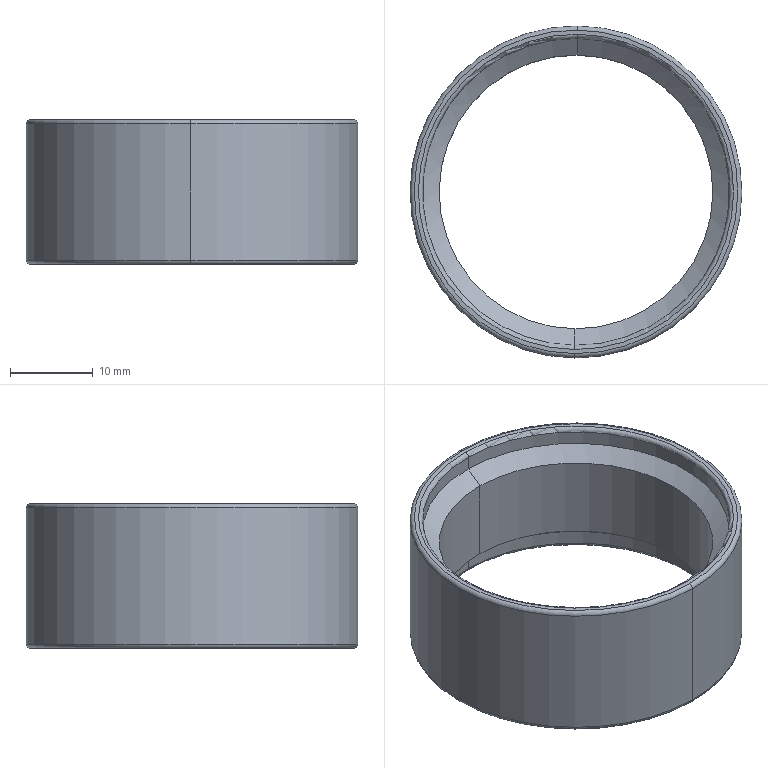Part | SolidWorks | features SplitBody 1 | 1 solid | 22 faces | box 40 x 40 x 17.4 mm | volume 5666 mm3 | cylinder 8 | torus 8 | cone 4 | plane 2 | commonest cylinder face diameters 37 x4 33 x2 40 x2
STEP:
#1=CARTESIAN_POINT('',(540.428,13.025,-486.947));
#2=VERTEX_POINT('',#1);
#3=CARTESIAN_POINT('',(540.156,-23.974,-486.947));
#4=VERTEX_POINT('',#3);
#5=CARTESIAN_POINT('',(540.292,-5.475,-486.947));
#6=DIRECTION('',(0.,0.,1.));
#7=DIRECTION('',(-0.00734,-1.,0.));
#8=AXIS2_PLACEMENT_3D('',#5,#6,#7);
#9=CIRCLE('',#8,18.5);
#10=EDGE_CURVE('',#2,#4,#9,.T.);
#11=ORIENTED_EDGE('',*,*,#10,.F.);
#12=CARTESIAN_POINT('',(540.428,13.025,-485.247));
#13=VERTEX_POINT('',#12);
#14=CARTESIAN_POINT('',(540.428,13.025,-478.747));
#15=DIRECTION('',(0.,0.,1.));
#16=VECTOR('',#15,1000.);
#17=LINE('',#14,#16);
#18=EDGE_CURVE('',#2,#13,#17,.T.);
#19=ORIENTED_EDGE('',*,*,#18,.T.);
#20=CARTESIAN_POINT('',(540.156,-23.974,-485.247));
#21=VERTEX_POINT('',#20);
#22=CARTESIAN_POINT('',(540.292,-5.475,-485.247));
#23=DIRECTION('',(0.,0.,1.));
#24=DIRECTION('',(-0.00734,-1.,0.));
#25=AXIS2_PLACEMENT_3D('',#22,#23,#24);
#26=CIRCLE('',#25,18.5);
#27=EDGE_CURVE('',#13,#21,#26,.T.);
#28=ORIENTED_EDGE('',*,*,#27,.T.);
#29=CARTESIAN_POINT('',(540.156,-23.974,-478.747));
#30=DIRECTION('',(0.,0.,1.));
#31=VECTOR('',#30,1000.);
#32=LINE('',#29,#31);
#33=EDGE_CURVE('',#4,#21,#32,.T.);
#34=ORIENTED_EDGE('',*,*,#33,.F.);
#35=EDGE_LOOP('',(#11,#19,#28,#34));
#36=FACE_OUTER_BOUND('',#35,.T.);
#37=CARTESIAN_POINT('',(540.292,-5.475,-478.747));
#38=DIRECTION('',(0.,0.,1.));
#39=DIRECTION('',(-0.00734,-1.,0.));
#40=AXIS2_PLACEMENT_3D('',#37,#38,#39);
#41=CYLINDRICAL_SURFACE('',#40,18.5);
#42=ADVANCED_FACE('',(#36),#41,.F.);
#43=CARTESIAN_POINT('',(540.292,-5.475,-486.947));
#44=DIRECTION('',(0.,0.,1.));
#45=DIRECTION('',(-0.00734,-1.,0.));
#46=AXIS2_PLACEMENT_3D('',#43,#44,#45);
#47=CIRCLE('',#46,18.5);
#48=EDGE_CURVE('',#4,#2,#47,.T.);
#49=ORIENTED_EDGE('',*,*,#48,.T.);
#50=CARTESIAN_POINT('',(540.432,13.525,-487.447));
#51=VERTEX_POINT('',#50);
#52=CARTESIAN_POINT('',(540.432,13.525,-486.947));
#53=DIRECTION('',(1.,-0.00734,0.));
#54=DIRECTION('',(0.00734,1.,0.));
#55=AXIS2_PLACEMENT_3D('',#52,#53,#54);
#56=CIRCLE('',#55,0.5);
#57=EDGE_CURVE('',#2,#51,#56,.T.);
#58=ORIENTED_EDGE('',*,*,#57,.T.);
#59=CARTESIAN_POINT('',(540.153,-24.474,-487.447));
#60=VERTEX_POINT('',#59);
#61=CARTESIAN_POINT('',(540.292,-5.475,-487.447));
#62=DIRECTION('',(0.,0.,1.));
#63=DIRECTION('',(-0.00734,-1.,0.));
#64=AXIS2_PLACEMENT_3D('',#61,#62,#63);
#65=CIRCLE('',#64,19.);
#66=EDGE_CURVE('',#60,#51,#65,.T.);
#67=ORIENTED_EDGE('',*,*,#66,.F.);
#68=CARTESIAN_POINT('',(540.153,-24.474,-486.947));
#69=DIRECTION('',(-1.,0.00734,0.));
#70=DIRECTION('',(-0.00734,-1.,0.));
#71=AXIS2_PLACEMENT_3D('',#68,#69,#70);
#72=CIRCLE('',#71,0.5);
#73=EDGE_CURVE('',#4,#60,#72,.T.);
#74=ORIENTED_EDGE('',*,*,#73,.F.);
#75=EDGE_LOOP('',(#49,#58,#67,#74));
#76=FACE_OUTER_BOUND('',#75,.T.);
#77=CARTESIAN_POINT('',(540.292,-5.475,-486.947));
#78=DIRECTION('',(0.,0.,1.));
#79=DIRECTION('',(-0.00734,-1.,0.));
#80=AXIS2_PLACEMENT_3D('',#77,#78,#79);
#81=TOROIDAL_SURFACE('',#80,19.,0.5);
#82=ADVANCED_FACE('',(#76),#81,.T.);
#83=CARTESIAN_POINT('',(540.149,-24.974,-487.447));
#84=VERTEX_POINT('',#83);
#85=CARTESIAN_POINT('',(540.435,14.025,-487.447));
#86=VERTEX_POINT('',#85);
#87=CARTESIAN_POINT('',(540.292,-5.475,-487.447));
#88=DIRECTION('',(0.,0.,1.));
#89=DIRECTION('',(-0.00734,-1.,0.));
#90=AXIS2_PLACEMENT_3D('',#87,#88,#89);
#91=CIRCLE('',#90,19.5);
#92=EDGE_CURVE('',#84,#86,#91,.T.);
#93=ORIENTED_EDGE('',*,*,#92,.T.);
#94=CARTESIAN_POINT('',(540.439,14.525,-486.947));
#95=VERTEX_POINT('',#94);
#96=CARTESIAN_POINT('',(540.435,14.025,-486.947));
#97=DIRECTION('',(1.,-0.00734,0.));
#98=DIRECTION('',(0.00734,1.,0.));
#99=AXIS2_PLACEMENT_3D('',#96,#97,#98);
#100=CIRCLE('',#99,0.5);
#101=EDGE_CURVE('',#86,#95,#100,.T.);
#102=ORIENTED_EDGE('',*,*,#101,.T.);
#103=CARTESIAN_POINT('',(540.145,-25.474,-486.947));
#104=VERTEX_POINT('',#103);
#105=CARTESIAN_POINT('',(540.292,-5.475,-486.947));
#106=DIRECTION('',(0.,0.,1.));
#107=DIRECTION('',(-0.00734,-1.,0.));
#108=AXIS2_PLACEMENT_3D('',#105,#106,#107);
#109=CIRCLE('',#108,20.);
#110=EDGE_CURVE('',#104,#95,#109,.T.);
#111=ORIENTED_EDGE('',*,*,#110,.F.);
#112=CARTESIAN_POINT('',(540.149,-24.974,-486.947));
#113=DIRECTION('',(-1.,0.00734,0.));
#114=DIRECTION('',(-0.00734,-1.,0.));
#115=AXIS2_PLACEMENT_3D('',#112,#113,#114);
#116=CIRCLE('',#115,0.5);
#117=EDGE_CURVE('',#84,#104,#116,.T.);
#118=ORIENTED_EDGE('',*,*,#117,.F.);
#119=EDGE_LOOP('',(#93,#102,#111,#118));
#120=FACE_OUTER_BOUND('',#119,.T.);
#121=CARTESIAN_POINT('',(540.292,-5.475,-486.947));
#122=DIRECTION('',(0.,0.,1.));
#123=DIRECTION('',(-0.00734,-1.,0.));
#124=AXIS2_PLACEMENT_3D('',#121,#122,#123);
#125=TOROIDAL_SURFACE('',#124,19.5,0.5);
#126=ADVANCED_FACE('',(#120),#125,.T.);
#127=ORIENTED_EDGE('',*,*,#110,.T.);
#128=CARTESIAN_POINT('',(540.439,14.525,-470.547));
#129=VERTEX_POINT('',#128);
#130=CARTESIAN_POINT('',(540.439,14.525,-478.747));
#131=DIRECTION('',(0.,0.,1.));
#132=VECTOR('',#131,1000.);
#133=LINE('',#130,#132);
#134=EDGE_CURVE('',#95,#129,#133,.T.);
#135=ORIENTED_EDGE('',*,*,#134,.T.);
#136=CARTESIAN_POINT('',(540.145,-25.474,-470.547));
#137=VERTEX_POINT('',#136);
#138=CARTESIAN_POINT('',(540.292,-5.475,-470.547));
#139=DIRECTION('',(0.,0.,1.));
#140=DIRECTION('',(-0.00734,-1.,0.));
#141=AXIS2_PLACEMENT_3D('',#138,#139,#140);
#142=CIRCLE('',#141,20.);
#143=EDGE_CURVE('',#137,#129,#142,.T.);
#144=ORIENTED_EDGE('',*,*,#143,.F.);
#145=CARTESIAN_POINT('',(540.145,-25.474,-478.747));
#146=DIRECTION('',(0.,0.,1.));
#147=VECTOR('',#146,1000.);
#148=LINE('',#145,#147);
#149=EDGE_CURVE('',#104,#137,#148,.T.);
#150=ORIENTED_EDGE('',*,*,#149,.F.);
#151=EDGE_LOOP('',(#127,#135,#144,#150));
#152=FACE_OUTER_BOUND('',#151,.T.);
#153=CARTESIAN_POINT('',(540.292,-5.475,-478.747));
#154=DIRECTION('',(0.,0.,1.));
#155=DIRECTION('',(-0.00734,-1.,0.));
#156=AXIS2_PLACEMENT_3D('',#153,#154,#155);
#157=CYLINDRICAL_SURFACE('',#156,20.);
#158=ADVANCED_FACE('',(#152),#157,.T.);
#159=ORIENTED_EDGE('',*,*,#143,.T.);
#160=CARTESIAN_POINT('',(540.435,14.025,-470.047));
#161=VERTEX_POINT('',#160);
#162=CARTESIAN_POINT('',(540.435,14.025,-470.547));
#163=DIRECTION('',(1.,-0.00734,0.));
#164=DIRECTION('',(0.00734,1.,0.));
#165=AXIS2_PLACEMENT_3D('',#162,#163,#164);
#166=CIRCLE('',#165,0.5);
#167=EDGE_CURVE('',#129,#161,#166,.T.);
#168=ORIENTED_EDGE('',*,*,#167,.T.);
#169=CARTESIAN_POINT('',(540.149,-24.974,-470.047));
#170=VERTEX_POINT('',#169);
#171=CARTESIAN_POINT('',(540.292,-5.475,-470.047));
#172=DIRECTION('',(0.,0.,1.));
#173=DIRECTION('',(-0.00734,-1.,0.));
#174=AXIS2_PLACEMENT_3D('',#171,#172,#173);
#175=CIRCLE('',#174,19.5);
#176=EDGE_CURVE('',#170,#161,#175,.T.);
#177=ORIENTED_EDGE('',*,*,#176,.F.);
#178=CARTESIAN_POINT('',(540.149,-24.974,-470.547));
#179=DIRECTION('',(-1.,0.00734,0.));
#180=DIRECTION('',(-0.00734,-1.,0.));
#181=AXIS2_PLACEMENT_3D('',#178,#179,#180);
#182=CIRCLE('',#181,0.5);
#183=EDGE_CURVE('',#137,#170,#182,.T.);
#184=ORIENTED_EDGE('',*,*,#183,.F.);
#185=EDGE_LOOP('',(#159,#168,#177,#184));
#186=FACE_OUTER_BOUND('',#185,.T.);
#187=CARTESIAN_POINT('',(540.292,-5.475,-470.547));
#188=DIRECTION('',(0.,0.,1.));
#189=DIRECTION('',(-0.00734,-1.,0.));
#190=AXIS2_PLACEMENT_3D('',#187,#188,#189);
#191=TOROIDAL_SURFACE('',#190,19.5,0.5);
#192=ADVANCED_FACE('',(#186),#191,.T.);
#193=CARTESIAN_POINT('',(540.153,-24.474,-470.047));
#194=VERTEX_POINT('',#193);
#195=CARTESIAN_POINT('',(540.432,13.525,-470.047));
#196=VERTEX_POINT('',#195);
#197=CARTESIAN_POINT('',(540.292,-5.475,-470.047));
#198=DIRECTION('',(0.,0.,1.));
#199=DIRECTION('',(-0.00734,-1.,0.));
#200=AXIS2_PLACEMENT_3D('',#197,#198,#199);
#201=CIRCLE('',#200,19.);
#202=EDGE_CURVE('',#194,#196,#201,.T.);
#203=ORIENTED_EDGE('',*,*,#202,.T.);
#204=CARTESIAN_POINT('',(540.428,13.025,-470.547));
#205=VERTEX_POINT('',#204);
#206=CARTESIAN_POINT('',(540.432,13.525,-470.547));
#207=DIRECTION('',(1.,-0.00734,0.));
#208=DIRECTION('',(0.00734,1.,0.));
#209=AXIS2_PLACEMENT_3D('',#206,#207,#208);
#210=CIRCLE('',#209,0.5);
#211=EDGE_CURVE('',#196,#205,#210,.T.);
#212=ORIENTED_EDGE('',*,*,#211,.T.);
#213=CARTESIAN_POINT('',(540.156,-23.974,-470.547));
#214=VERTEX_POINT('',#213);
#215=CARTESIAN_POINT('',(540.292,-5.475,-470.547));
#216=DIRECTION('',(0.,0.,1.));
#217=DIRECTION('',(-0.00734,-1.,0.));
#218=AXIS2_PLACEMENT_3D('',#215,#216,#217);
#219=CIRCLE('',#218,18.5);
#220=EDGE_CURVE('',#214,#205,#219,.T.);
#221=ORIENTED_EDGE('',*,*,#220,.F.);
#222=CARTESIAN_POINT('',(540.153,-24.474,-470.547));
#223=DIRECTION('',(-1.,0.00734,0.));
#224=DIRECTION('',(-0.00734,-1.,0.));
#225=AXIS2_PLACEMENT_3D('',#222,#223,#224);
#226=CIRCLE('',#225,0.5);
#227=EDGE_CURVE('',#194,#214,#226,.T.);
#228=ORIENTED_EDGE('',*,*,#227,.F.);
#229=EDGE_LOOP('',(#203,#212,#221,#228));
#230=FACE_OUTER_BOUND('',#229,.T.);
#231=CARTESIAN_POINT('',(540.292,-5.475,-470.547));
#232=DIRECTION('',(0.,0.,1.));
#233=DIRECTION('',(-0.00734,-1.,0.));
#234=AXIS2_PLACEMENT_3D('',#231,#232,#233);
#235=TOROIDAL_SURFACE('',#234,19.,0.5);
#236=ADVANCED_FACE('',(#230),#235,.T.);
#237=CARTESIAN_POINT('',(540.428,13.025,-472.247));
#238=VERTEX_POINT('',#237);
#239=CARTESIAN_POINT('',(540.156,-23.974,-472.247));
#240=VERTEX_POINT('',#239);
#241=CARTESIAN_POINT('',(540.292,-5.475,-472.247));
#242=DIRECTION('',(0.,0.,1.));
#243=DIRECTION('',(-0.00734,-1.,0.));
#244=AXIS2_PLACEMENT_3D('',#241,#242,#243);
#245=CIRCLE('',#244,18.5);
#246=EDGE_CURVE('',#238,#240,#245,.T.);
#247=ORIENTED_EDGE('',*,*,#246,.F.);
#248=CARTESIAN_POINT('',(540.428,13.025,-478.747));
#249=DIRECTION('',(0.,0.,1.));
#250=VECTOR('',#249,1000.);
#251=LINE('',#248,#250);
#252=EDGE_CURVE('',#238,#205,#251,.T.);
#253=ORIENTED_EDGE('',*,*,#252,.T.);
#254=CARTESIAN_POINT('',(540.292,-5.475,-470.547));
#255=DIRECTION('',(0.,0.,1.));
#256=DIRECTION('',(-0.00734,-1.,0.));
#257=AXIS2_PLACEMENT_3D('',#254,#255,#256);
#258=CIRCLE('',#257,18.5);
#259=EDGE_CURVE('',#205,#214,#258,.T.);
#260=ORIENTED_EDGE('',*,*,#259,.T.);
#261=CARTESIAN_POINT('',(540.156,-23.974,-478.747));
#262=DIRECTION('',(0.,0.,1.));
#263=VECTOR('',#262,1000.);
#264=LINE('',#261,#263);
#265=EDGE_CURVE('',#240,#214,#264,.T.);
#266=ORIENTED_EDGE('',*,*,#265,.F.);
#267=EDGE_LOOP('',(#247,#253,#260,#266));
#268=FACE_OUTER_BOUND('',#267,.T.);
#269=CARTESIAN_POINT('',(540.292,-5.475,-478.747));
#270=DIRECTION('',(0.,0.,1.));
#271=DIRECTION('',(-0.00734,-1.,0.));
#272=AXIS2_PLACEMENT_3D('',#269,#270,#271);
#273=CYLINDRICAL_SURFACE('',#272,18.5);
#274=ADVANCED_FACE('',(#268),#273,.F.);
#275=CARTESIAN_POINT('',(540.413,11.025,-473.747));
#276=VERTEX_POINT('',#275);
#277=CARTESIAN_POINT('',(540.171,-21.974,-473.747));
#278=VERTEX_POINT('',#277);
#279=CARTESIAN_POINT('',(540.292,-5.475,-473.747));
#280=DIRECTION('',(0.,0.,1.));
#281=DIRECTION('',(-0.00734,-1.,0.));
#282=AXIS2_PLACEMENT_3D('',#279,#280,#281);
#283=CIRCLE('',#282,16.5);
#284=EDGE_CURVE('',#276,#278,#283,.T.);
#285=ORIENTED_EDGE('',*,*,#284,.F.);
#286=CARTESIAN_POINT('',(540.413,11.025,-473.747));
#287=DIRECTION('',(0.005872,0.8,0.6));
#288=VECTOR('',#287,1000.);
#289=LINE('',#286,#288);
#290=EDGE_CURVE('',#276,#238,#289,.T.);
#291=ORIENTED_EDGE('',*,*,#290,.T.);
#292=ORIENTED_EDGE('',*,*,#246,.T.);
#293=CARTESIAN_POINT('',(540.171,-21.974,-473.747));
#294=DIRECTION('',(-0.005872,-0.8,0.6));
#295=VECTOR('',#294,1000.);
#296=LINE('',#293,#295);
#297=EDGE_CURVE('',#278,#240,#296,.T.);
#298=ORIENTED_EDGE('',*,*,#297,.F.);
#299=EDGE_LOOP('',(#285,#291,#292,#298));
#300=FACE_OUTER_BOUND('',#299,.T.);
#301=CARTESIAN_POINT('',(540.292,-5.475,-473.747));
#302=DIRECTION('',(0.,0.,1.));
#303=DIRECTION('',(-0.00734,-1.,0.));
#304=AXIS2_PLACEMENT_3D('',#301,#302,#303);
#305=CONICAL_SURFACE('',#304,16.5,0.9273);
#306=ADVANCED_FACE('',(#300),#305,.F.);
#307=CARTESIAN_POINT('',(540.413,11.025,-483.747));
#308=VERTEX_POINT('',#307);
#309=CARTESIAN_POINT('',(540.171,-21.974,-483.747));
#310=VERTEX_POINT('',#309);
#311=CARTESIAN_POINT('',(540.292,-5.475,-483.747));
#312=DIRECTION('',(0.,0.,1.));
#313=DIRECTION('',(-0.00734,-1.,0.));
#314=AXIS2_PLACEMENT_3D('',#311,#312,#313);
#315=CIRCLE('',#314,16.5);
#316=EDGE_CURVE('',#308,#310,#315,.T.);
#317=ORIENTED_EDGE('',*,*,#316,.F.);
#318=CARTESIAN_POINT('',(540.413,11.025,-478.747));
#319=DIRECTION('',(0.,0.,1.));
#320=VECTOR('',#319,1000.);
#321=LINE('',#318,#320);
#322=EDGE_CURVE('',#308,#276,#321,.T.);
#323=ORIENTED_EDGE('',*,*,#322,.T.);
#324=ORIENTED_EDGE('',*,*,#284,.T.);
#325=CARTESIAN_POINT('',(540.171,-21.974,-478.747));
#326=DIRECTION('',(0.,0.,1.));
#327=VECTOR('',#326,1000.);
#328=LINE('',#325,#327);
#329=EDGE_CURVE('',#310,#278,#328,.T.);
#330=ORIENTED_EDGE('',*,*,#329,.F.);
#331=EDGE_LOOP('',(#317,#323,#324,#330));
#332=FACE_OUTER_BOUND('',#331,.T.);
#333=CARTESIAN_POINT('',(540.292,-5.475,-478.747));
#334=DIRECTION('',(0.,0.,1.));
#335=DIRECTION('',(-0.00734,-1.,0.));
#336=AXIS2_PLACEMENT_3D('',#333,#334,#335);
#337=CYLINDRICAL_SURFACE('',#336,16.5);
#338=ADVANCED_FACE('',(#332),#337,.F.);
#339=ORIENTED_EDGE('',*,*,#316,.T.);
#340=CARTESIAN_POINT('',(540.156,-23.974,-485.247));
#341=DIRECTION('',(-0.005872,-0.8,-0.6));
#342=VECTOR('',#341,1000.);
#343=LINE('',#340,#342);
#344=EDGE_CURVE('',#310,#21,#343,.T.);
#345=ORIENTED_EDGE('',*,*,#344,.T.);
#346=ORIENTED_EDGE('',*,*,#27,.F.);
#347=CARTESIAN_POINT('',(540.428,13.025,-485.247));
#348=DIRECTION('',(0.005872,0.8,-0.6));
#349=VECTOR('',#348,1000.);
#350=LINE('',#347,#349);
#351=EDGE_CURVE('',#308,#13,#350,.T.);
#352=ORIENTED_EDGE('',*,*,#351,.F.);
#353=EDGE_LOOP('',(#339,#345,#346,#352));
#354=FACE_OUTER_BOUND('',#353,.T.);
#355=CARTESIAN_POINT('',(540.292,-5.475,-485.247));
#356=DIRECTION('',(0.,0.,-1.));
#357=DIRECTION('',(0.00734,1.,0.));
#358=AXIS2_PLACEMENT_3D('',#355,#356,#357);
#359=CONICAL_SURFACE('',#358,18.5,0.9273);
#360=ADVANCED_FACE('',(#354),#359,.F.);
#361=ORIENTED_EDGE('',*,*,#344,.F.);
#362=CARTESIAN_POINT('',(540.292,-5.475,-483.747));
#363=DIRECTION('',(0.,0.,1.));
#364=DIRECTION('',(-0.00734,-1.,0.));
#365=AXIS2_PLACEMENT_3D('',#362,#363,#364);
#366=CIRCLE('',#365,16.5);
#367=EDGE_CURVE('',#310,#308,#366,.T.);
#368=ORIENTED_EDGE('',*,*,#367,.T.);
#369=ORIENTED_EDGE('',*,*,#351,.T.);
#370=CARTESIAN_POINT('',(540.292,-5.475,-485.247));
#371=DIRECTION('',(0.,0.,1.));
#372=DIRECTION('',(-0.00734,-1.,0.));
#373=AXIS2_PLACEMENT_3D('',#370,#371,#372);
#374=CIRCLE('',#373,18.5);
#375=EDGE_CURVE('',#21,#13,#374,.T.);
#376=ORIENTED_EDGE('',*,*,#375,.F.);
#377=EDGE_LOOP('',(#361,#368,#369,#376));
#378=FACE_OUTER_BOUND('',#377,.T.);
#379=CARTESIAN_POINT('',(540.292,-5.475,-485.247));
#380=DIRECTION('',(0.,0.,-1.));
#381=DIRECTION('',(0.00734,1.,0.));
#382=AXIS2_PLACEMENT_3D('',#379,#380,#381);
#383=CONICAL_SURFACE('',#382,18.5,0.9273);
#384=ADVANCED_FACE('',(#378),#383,.F.);
#385=ORIENTED_EDGE('',*,*,#322,.F.);
#386=ORIENTED_EDGE('',*,*,#367,.F.);
#387=ORIENTED_EDGE('',*,*,#329,.T.);
#388=CARTESIAN_POINT('',(540.292,-5.475,-473.747));
#389=DIRECTION('',(0.,0.,1.));
#390=DIRECTION('',(-0.00734,-1.,0.));
#391=AXIS2_PLACEMENT_3D('',#388,#389,#390);
#392=CIRCLE('',#391,16.5);
#393=EDGE_CURVE('',#278,#276,#392,.T.);
#394=ORIENTED_EDGE('',*,*,#393,.T.);
#395=EDGE_LOOP('',(#385,#386,#387,#394));
#396=FACE_OUTER_BOUND('',#395,.T.);
#397=CARTESIAN_POINT('',(540.292,-5.475,-478.747));
#398=DIRECTION('',(0.,0.,1.));
#399=DIRECTION('',(-0.00734,-1.,0.));
#400=AXIS2_PLACEMENT_3D('',#397,#398,#399);
#401=CYLINDRICAL_SURFACE('',#400,16.5);
#402=ADVANCED_FACE('',(#396),#401,.F.);
#403=ORIENTED_EDGE('',*,*,#290,.F.);
#404=ORIENTED_EDGE('',*,*,#393,.F.);
#405=ORIENTED_EDGE('',*,*,#297,.T.);
#406=CARTESIAN_POINT('',(540.292,-5.475,-472.247));
#407=DIRECTION('',(0.,0.,1.));
#408=DIRECTION('',(-0.00734,-1.,0.));
#409=AXIS2_PLACEMENT_3D('',#406,#407,#408);
#410=CIRCLE('',#409,18.5);
#411=EDGE_CURVE('',#240,#238,#410,.T.);
#412=ORIENTED_EDGE('',*,*,#411,.T.);
#413=EDGE_LOOP('',(#403,#404,#405,#412));
#414=FACE_OUTER_BOUND('',#413,.T.);
#415=CARTESIAN_POINT('',(540.292,-5.475,-473.747));
#416=DIRECTION('',(0.,0.,1.));
#417=DIRECTION('',(-0.00734,-1.,0.));
#418=AXIS2_PLACEMENT_3D('',#415,#416,#417);
#419=CONICAL_SURFACE('',#418,16.5,0.9273);
#420=ADVANCED_FACE('',(#414),#419,.F.);
#421=ORIENTED_EDGE('',*,*,#252,.F.);
#422=ORIENTED_EDGE('',*,*,#411,.F.);
#423=ORIENTED_EDGE('',*,*,#265,.T.);
#424=ORIENTED_EDGE('',*,*,#220,.T.);
#425=EDGE_LOOP('',(#421,#422,#423,#424));
#426=FACE_OUTER_BOUND('',#425,.T.);
#427=CARTESIAN_POINT('',(540.292,-5.475,-478.747));
#428=DIRECTION('',(0.,0.,1.));
#429=DIRECTION('',(-0.00734,-1.,0.));
#430=AXIS2_PLACEMENT_3D('',#427,#428,#429);
#431=CYLINDRICAL_SURFACE('',#430,18.5);
#432=ADVANCED_FACE('',(#426),#431,.F.);
#433=ORIENTED_EDGE('',*,*,#211,.F.);
#434=CARTESIAN_POINT('',(540.292,-5.475,-470.047));
#435=DIRECTION('',(0.,0.,1.));
#436=DIRECTION('',(-0.00734,-1.,0.));
#437=AXIS2_PLACEMENT_3D('',#434,#435,#436);
#438=CIRCLE('',#437,19.);
#439=EDGE_CURVE('',#196,#194,#438,.T.);
#440=ORIENTED_EDGE('',*,*,#439,.T.);
#441=ORIENTED_EDGE('',*,*,#227,.T.);
#442=ORIENTED_EDGE('',*,*,#259,.F.);
#443=EDGE_LOOP('',(#433,#440,#441,#442));
#444=FACE_OUTER_BOUND('',#443,.T.);
#445=CARTESIAN_POINT('',(540.292,-5.475,-470.547));
#446=DIRECTION('',(0.,0.,1.));
#447=DIRECTION('',(-0.00734,-1.,0.));
#448=AXIS2_PLACEMENT_3D('',#445,#446,#447);
#449=TOROIDAL_SURFACE('',#448,19.,0.5);
#450=ADVANCED_FACE('',(#444),#449,.T.);
#451=ORIENTED_EDGE('',*,*,#176,.T.);
#452=CARTESIAN_POINT('',(540.292,-5.475,-470.047));
#453=DIRECTION('',(0.,0.,1.));
#454=DIRECTION('',(-0.00734,-1.,0.));
#455=AXIS2_PLACEMENT_3D('',#452,#453,#454);
#456=CIRCLE('',#455,19.5);
#457=EDGE_CURVE('',#161,#170,#456,.T.);
#458=ORIENTED_EDGE('',*,*,#457,.T.);
#459=EDGE_LOOP('',(#451,#458));
#460=FACE_OUTER_BOUND('',#459,.T.);
#461=ORIENTED_EDGE('',*,*,#202,.F.);
#462=ORIENTED_EDGE('',*,*,#439,.F.);
#463=EDGE_LOOP('',(#461,#462));
#464=FACE_BOUND('',#463,.T.);
#465=CARTESIAN_POINT('',(559.292,-5.614,-470.047));
#466=DIRECTION('',(0.,0.,1.));
#467=DIRECTION('',(-0.00734,-1.,0.));
#468=AXIS2_PLACEMENT_3D('',#465,#466,#467);
#469=PLANE('',#468);
#470=ADVANCED_FACE('',(#460,#464),#469,.T.);
#471=ORIENTED_EDGE('',*,*,#167,.F.);
#472=CARTESIAN_POINT('',(540.292,-5.475,-470.547));
#473=DIRECTION('',(0.,0.,1.));
#474=DIRECTION('',(-0.00734,-1.,0.));
#475=AXIS2_PLACEMENT_3D('',#472,#473,#474);
#476=CIRCLE('',#475,20.);
#477=EDGE_CURVE('',#129,#137,#476,.T.);
#478=ORIENTED_EDGE('',*,*,#477,.T.);
#479=ORIENTED_EDGE('',*,*,#183,.T.);
#480=ORIENTED_EDGE('',*,*,#457,.F.);
#481=EDGE_LOOP('',(#471,#478,#479,#480));
#482=FACE_OUTER_BOUND('',#481,.T.);
#483=CARTESIAN_POINT('',(540.292,-5.475,-470.547));
#484=DIRECTION('',(0.,0.,1.));
#485=DIRECTION('',(-0.00734,-1.,0.));
#486=AXIS2_PLACEMENT_3D('',#483,#484,#485);
#487=TOROIDAL_SURFACE('',#486,19.5,0.5);
#488=ADVANCED_FACE('',(#482),#487,.T.);
#489=ORIENTED_EDGE('',*,*,#134,.F.);
#490=CARTESIAN_POINT('',(540.292,-5.475,-486.947));
#491=DIRECTION('',(0.,0.,1.));
#492=DIRECTION('',(-0.00734,-1.,0.));
#493=AXIS2_PLACEMENT_3D('',#490,#491,#492);
#494=CIRCLE('',#493,20.);
#495=EDGE_CURVE('',#95,#104,#494,.T.);
#496=ORIENTED_EDGE('',*,*,#495,.T.);
#497=ORIENTED_EDGE('',*,*,#149,.T.);
#498=ORIENTED_EDGE('',*,*,#477,.F.);
#499=EDGE_LOOP('',(#489,#496,#497,#498));
#500=FACE_OUTER_BOUND('',#499,.T.);
#501=CARTESIAN_POINT('',(540.292,-5.475,-478.747));
#502=DIRECTION('',(0.,0.,1.));
#503=DIRECTION('',(-0.00734,-1.,0.));
#504=AXIS2_PLACEMENT_3D('',#501,#502,#503);
#505=CYLINDRICAL_SURFACE('',#504,20.);
#506=ADVANCED_FACE('',(#500),#505,.T.);
#507=ORIENTED_EDGE('',*,*,#101,.F.);
#508=CARTESIAN_POINT('',(540.292,-5.475,-487.447));
#509=DIRECTION('',(0.,0.,1.));
#510=DIRECTION('',(-0.00734,-1.,0.));
#511=AXIS2_PLACEMENT_3D('',#508,#509,#510);
#512=CIRCLE('',#511,19.5);
#513=EDGE_CURVE('',#86,#84,#512,.T.);
#514=ORIENTED_EDGE('',*,*,#513,.T.);
#515=ORIENTED_EDGE('',*,*,#117,.T.);
#516=ORIENTED_EDGE('',*,*,#495,.F.);
#517=EDGE_LOOP('',(#507,#514,#515,#516));
#518=FACE_OUTER_BOUND('',#517,.T.);
#519=CARTESIAN_POINT('',(540.292,-5.475,-486.947));
#520=DIRECTION('',(0.,0.,1.));
#521=DIRECTION('',(-0.00734,-1.,0.));
#522=AXIS2_PLACEMENT_3D('',#519,#520,#521);
#523=TOROIDAL_SURFACE('',#522,19.5,0.5);
#524=ADVANCED_FACE('',(#518),#523,.T.);
#525=ORIENTED_EDGE('',*,*,#66,.T.);
#526=CARTESIAN_POINT('',(540.292,-5.475,-487.447));
#527=DIRECTION('',(0.,0.,1.));
#528=DIRECTION('',(-0.00734,-1.,0.));
#529=AXIS2_PLACEMENT_3D('',#526,#527,#528);
#530=CIRCLE('',#529,19.);
#531=EDGE_CURVE('',#51,#60,#530,.T.);
#532=ORIENTED_EDGE('',*,*,#531,.T.);
#533=EDGE_LOOP('',(#525,#532));
#534=FACE_BOUND('',#533,.T.);
#535=ORIENTED_EDGE('',*,*,#92,.F.);
#536=ORIENTED_EDGE('',*,*,#513,.F.);
#537=EDGE_LOOP('',(#535,#536));
#538=FACE_OUTER_BOUND('',#537,.T.);
#539=CARTESIAN_POINT('',(559.792,-5.618,-487.447));
#540=DIRECTION('',(0.,0.,-1.));
#541=DIRECTION('',(0.00734,1.,0.));
#542=AXIS2_PLACEMENT_3D('',#539,#540,#541);
#543=PLANE('',#542);
#544=ADVANCED_FACE('',(#534,#538),#543,.T.);
#545=ORIENTED_EDGE('',*,*,#57,.F.);
#546=ORIENTED_EDGE('',*,*,#10,.T.);
#547=ORIENTED_EDGE('',*,*,#73,.T.);
#548=ORIENTED_EDGE('',*,*,#531,.F.);
#549=EDGE_LOOP('',(#545,#546,#547,#548));
#550=FACE_OUTER_BOUND('',#549,.T.);
#551=CARTESIAN_POINT('',(540.292,-5.475,-486.947));
#552=DIRECTION('',(0.,0.,1.));
#553=DIRECTION('',(-0.00734,-1.,0.));
#554=AXIS2_PLACEMENT_3D('',#551,#552,#553);
#555=TOROIDAL_SURFACE('',#554,19.,0.5);
#556=ADVANCED_FACE('',(#550),#555,.T.);
#557=ORIENTED_EDGE('',*,*,#18,.F.);
#558=ORIENTED_EDGE('',*,*,#48,.F.);
#559=ORIENTED_EDGE('',*,*,#33,.T.);
#560=ORIENTED_EDGE('',*,*,#375,.T.);
#561=EDGE_LOOP('',(#557,#558,#559,#560));
#562=FACE_OUTER_BOUND('',#561,.T.);
#563=CARTESIAN_POINT('',(540.292,-5.475,-478.747));
#564=DIRECTION('',(0.,0.,1.));
#565=DIRECTION('',(-0.00734,-1.,0.));
#566=AXIS2_PLACEMENT_3D('',#563,#564,#565);
#567=CYLINDRICAL_SURFACE('',#566,18.5);
#568=ADVANCED_FACE('',(#562),#567,.F.);
#569=CLOSED_SHELL('',(#42,#82,#126,#158,#192,#236,#274,#306,#338,#360,#384,#402,#420,#432,#450,#470,#488,#506,#524,#544,#556,#568));
#570=MANIFOLD_SOLID_BREP('',#569);
#571=CARTESIAN_POINT('',(0.,0.,0.));
#572=DIRECTION('',(0.,0.,1.));
#573=DIRECTION('',(1.,0.,0.));
#574=AXIS2_PLACEMENT_3D('',#571,#572,#573);
#575=(LENGTH_UNIT()NAMED_UNIT(*)SI_UNIT(.MILLI.,.METRE.));
#576=UNCERTAINTY_MEASURE_WITH_UNIT(LENGTH_MEASURE(0.00001),#575,'','');
#577=(NAMED_UNIT(*)PLANE_ANGLE_UNIT()SI_UNIT($,.RADIAN.));
#578=(NAMED_UNIT(*)SI_UNIT($,.STERADIAN.)SOLID_ANGLE_UNIT());
#579=(GEOMETRIC_REPRESENTATION_CONTEXT(3)GLOBAL_UNCERTAINTY_ASSIGNED_CONTEXT((#576))GLOBAL_UNIT_ASSIGNED_CONTEXT((#575,#577,#578))REPRESENTATION_CONTEXT('',''));
#580=ADVANCED_BREP_SHAPE_REPRESENTATION('',(#570,#574),#579);